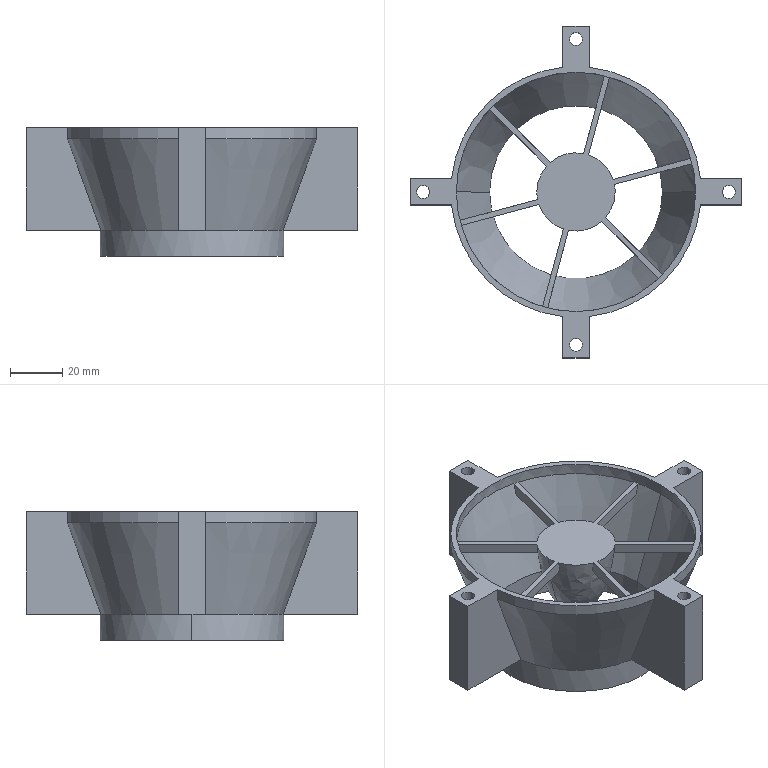Part | SolidWorks | features ICE 8, CirPattern 2, Revolution 2, Shell 1 | 1 solid | 63 faces | box 127.2 x 127.2 x 49.3 mm | volume 72395 mm3 | plane 37 | cylinder 18 | cone 6 | spline 2 | commonest cylinder face diameters 5 x8 96 x4 66.265 x2 70.522 x2 91.743 x2